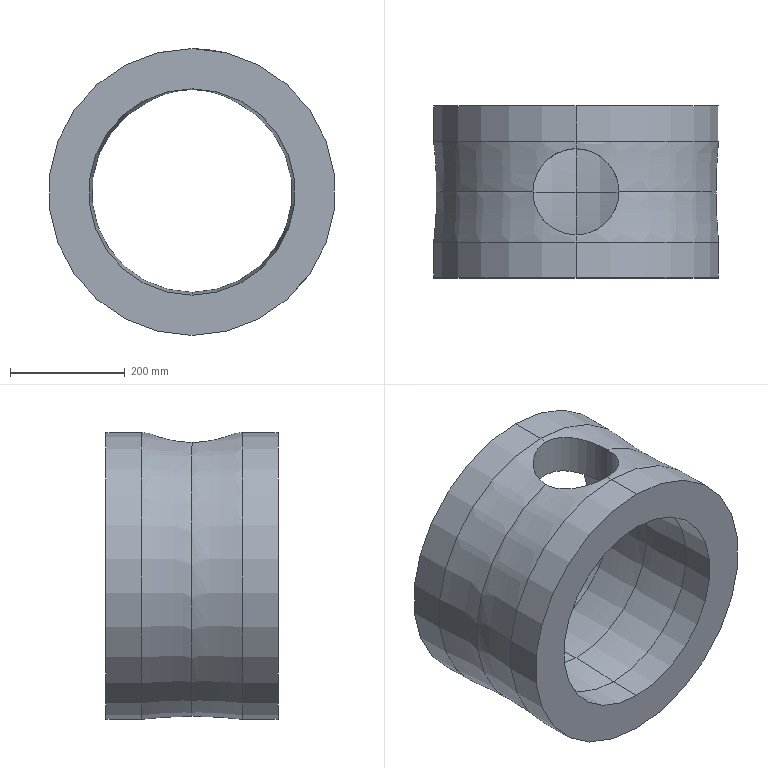Part | SolidWorks | features ICE 1, Revolution 1, Shell 1 | 1 solid | 20 faces | box 500 x 300 x 500 mm | volume 26874622 mm3 | cylinder 10 | torus 8 | plane 2 | commonest cylinder face diameters 360 x4 500 x4 150 x2
STEP:
#1=CARTESIAN_POINT('',(-75.,150.,157.967));
#2=VERTEX_POINT('',#1);
#3=CARTESIAN_POINT('',(0.,225.,178.283));
#4=VERTEX_POINT('',#3);
#5=CARTESIAN_POINT('',(-75.,150.,157.967));
#6=CARTESIAN_POINT('',(-75.,154.992,157.967));
#7=CARTESIAN_POINT('',(-74.507,159.931,158.255));
#8=CARTESIAN_POINT('',(-73.398,165.431,158.877));
#9=CARTESIAN_POINT('',(-73.267,166.041,158.95));
#10=CARTESIAN_POINT('',(-72.99,167.26,159.105));
#11=CARTESIAN_POINT('',(-72.843,167.869,159.186));
#12=CARTESIAN_POINT('',(-72.382,169.683,159.441));
#13=CARTESIAN_POINT('',(-72.046,170.877,159.626));
#14=CARTESIAN_POINT('',(-70.956,174.421,160.219));
#15=CARTESIAN_POINT('',(-70.119,176.728,160.667));
#16=CARTESIAN_POINT('',(-68.229,181.238,161.65));
#17=CARTESIAN_POINT('',(-67.176,183.442,162.186));
#18=CARTESIAN_POINT('',(-65.435,186.671,163.043));
#19=CARTESIAN_POINT('',(-64.826,187.737,163.338));
#20=CARTESIAN_POINT('',(-63.563,189.827,163.939));
#21=CARTESIAN_POINT('',(-62.909,190.852,164.245));
#22=CARTESIAN_POINT('',(-60.881,193.868,165.176));
#23=CARTESIAN_POINT('',(-59.44,195.801,165.814));
#24=CARTESIAN_POINT('',(-56.381,199.518,167.105));
#25=CARTESIAN_POINT('',(-54.763,201.302,167.76));
#26=CARTESIAN_POINT('',(-52.2,203.867,168.74));
#27=CARTESIAN_POINT('',(-51.323,204.703,169.067));
#28=CARTESIAN_POINT('',(-49.521,206.339,169.718));
#29=CARTESIAN_POINT('',(-48.601,207.135,170.041));
#30=CARTESIAN_POINT('',(-45.795,209.445,170.995));
#31=CARTESIAN_POINT('',(-43.859,210.887,171.613));
#32=CARTESIAN_POINT('',(-39.853,213.581,172.796));
#33=CARTESIAN_POINT('',(-37.784,214.833,173.362));
#34=CARTESIAN_POINT('',(-33.507,217.143,174.428));
#35=CARTESIAN_POINT('',(-31.299,218.202,174.928));
#36=CARTESIAN_POINT('',(-28.446,219.399,175.502));
#37=CARTESIAN_POINT('',(-27.87,219.632,175.614));
#38=CARTESIAN_POINT('',(-26.715,220.084,175.833));
#39=CARTESIAN_POINT('',(-26.135,220.302,175.938));
#40=CARTESIAN_POINT('',(-24.391,220.934,176.247));
#41=CARTESIAN_POINT('',(-23.22,221.326,176.439));
#42=CARTESIAN_POINT('',(-19.684,222.413,176.976));
#43=CARTESIAN_POINT('',(-17.296,223.02,177.28));
#44=CARTESIAN_POINT('',(-12.458,223.999,177.773));
#45=CARTESIAN_POINT('',(-10.008,224.371,177.962));
#46=CARTESIAN_POINT('',(-6.284,224.747,178.154));
#47=CARTESIAN_POINT('',(-5.034,224.841,178.202));
#48=CARTESIAN_POINT('',(-3.147,224.937,178.251));
#49=CARTESIAN_POINT('',(-2.516,224.96,178.263));
#50=CARTESIAN_POINT('',(-1.256,224.992,178.279));
#51=CARTESIAN_POINT('',(-0.6274,225.,178.283));
#52=CARTESIAN_POINT('',(0.,225.,178.283));
#53=B_SPLINE_CURVE_WITH_KNOTS('',3,(#5,#6,#7,#8,#9,#10,#11,#12,#13,#14,#15,#16,#17,#18,#19,#20,#21,#22,#23,#24,#25,#26,#27,#28,#29,#30,#31,#32,#33,#34,#35,#36,#37,#38,#39,#40,#41,#42,#43,#44,#45,#46,#47,#48,#49,#50,#51,#52),.UNSPECIFIED.,.F.,.F.,(4,2,2,2,2,2,2,2,2,2,2,2,2,2,2,2,2,2,2,2,2,2,2,4),(0.05661,0.07153,0.0734,0.07526,0.07899,0.08645,0.09392,0.09765,0.1014,0.1088,0.1163,0.12,0.1238,0.1312,0.1387,0.1461,0.148,0.1499,0.1536,0.1611,0.1685,0.1723,0.1741,0.176),.UNSPECIFIED.);
#54=EDGE_CURVE('',#2,#4,#53,.T.);
#55=ORIENTED_EDGE('',*,*,#54,.F.);
#56=CARTESIAN_POINT('',(0.,150.,-174.868));
#57=VERTEX_POINT('',#56);
#58=CARTESIAN_POINT('',(0.,150.,0.));
#59=DIRECTION('',(0.,-1.,0.));
#60=DIRECTION('',(0.,0.,-1.));
#61=AXIS2_PLACEMENT_3D('',#58,#59,#60);
#62=CIRCLE('',#61,174.868);
#63=EDGE_CURVE('',#2,#57,#62,.T.);
#64=ORIENTED_EDGE('',*,*,#63,.T.);
#65=CARTESIAN_POINT('',(0.,241.887,-180.));
#66=VERTEX_POINT('',#65);
#67=CARTESIAN_POINT('',(0.,150.,-1000.));
#68=DIRECTION('',(-1.,0.,0.));
#69=DIRECTION('',(0.,0.,1.));
#70=AXIS2_PLACEMENT_3D('',#67,#68,#69);
#71=CIRCLE('',#70,825.132);
#72=EDGE_CURVE('',#57,#66,#71,.T.);
#73=ORIENTED_EDGE('',*,*,#72,.T.);
#74=CARTESIAN_POINT('',(0.,241.887,180.));
#75=VERTEX_POINT('',#74);
#76=CARTESIAN_POINT('',(0.,241.887,0.));
#77=DIRECTION('',(0.,-1.,0.));
#78=DIRECTION('',(0.,0.,-1.));
#79=AXIS2_PLACEMENT_3D('',#76,#77,#78);
#80=CIRCLE('',#79,180.);
#81=EDGE_CURVE('',#75,#66,#80,.T.);
#82=ORIENTED_EDGE('',*,*,#81,.F.);
#83=CARTESIAN_POINT('',(0.,150.,1000.));
#84=DIRECTION('',(1.,0.,0.));
#85=DIRECTION('',(0.,0.,-1.));
#86=AXIS2_PLACEMENT_3D('',#83,#84,#85);
#87=CIRCLE('',#86,825.132);
#88=EDGE_CURVE('',#4,#75,#87,.T.);
#89=ORIENTED_EDGE('',*,*,#88,.F.);
#90=EDGE_LOOP('',(#55,#64,#73,#82,#89));
#91=FACE_OUTER_BOUND('',#90,.T.);
#92=CARTESIAN_POINT('',(0.,150.,0.));
#93=DIRECTION('',(0.,-1.,0.));
#94=DIRECTION('',(0.,0.,-1.));
#95=AXIS2_PLACEMENT_3D('',#92,#93,#94);
#96=TOROIDAL_SURFACE('',#95,1000.,825.132);
#97=ADVANCED_FACE('',(#91),#96,.T.);
#98=CARTESIAN_POINT('',(0.,62.11,-250.));
#99=VERTEX_POINT('',#98);
#100=CARTESIAN_POINT('',(0.,150.,-244.868));
#101=VERTEX_POINT('',#100);
#102=CARTESIAN_POINT('',(0.,150.,-1000.));
#103=DIRECTION('',(-1.,0.,0.));
#104=DIRECTION('',(0.,0.,1.));
#105=AXIS2_PLACEMENT_3D('',#102,#103,#104);
#106=CIRCLE('',#105,755.132);
#107=EDGE_CURVE('',#99,#101,#106,.T.);
#108=ORIENTED_EDGE('',*,*,#107,.T.);
#109=CARTESIAN_POINT('',(75.,150.,233.099));
#110=VERTEX_POINT('',#109);
#111=CARTESIAN_POINT('',(0.,150.,0.));
#112=DIRECTION('',(0.,-1.,0.));
#113=DIRECTION('',(0.,0.,-1.));
#114=AXIS2_PLACEMENT_3D('',#111,#112,#113);
#115=CIRCLE('',#114,244.868);
#116=EDGE_CURVE('',#101,#110,#115,.T.);
#117=ORIENTED_EDGE('',*,*,#116,.T.);
#118=CARTESIAN_POINT('',(0.,75.,248.601));
#119=VERTEX_POINT('',#118);
#120=CARTESIAN_POINT('',(75.,150.,233.099));
#121=CARTESIAN_POINT('',(75.,148.76,233.099));
#122=CARTESIAN_POINT('',(74.969,147.517,233.112));
#123=CARTESIAN_POINT('',(74.876,145.647,233.152));
#124=CARTESIAN_POINT('',(74.837,145.021,233.168));
#125=CARTESIAN_POINT('',(74.744,143.775,233.208));
#126=CARTESIAN_POINT('',(74.689,143.153,233.231));
#127=CARTESIAN_POINT('',(74.38,140.057,233.362));
#128=CARTESIAN_POINT('',(74.011,137.612,233.518));
#129=CARTESIAN_POINT('',(73.039,132.784,233.923));
#130=CARTESIAN_POINT('',(72.436,130.4,234.172));
#131=CARTESIAN_POINT('',(71.355,126.871,234.61));
#132=CARTESIAN_POINT('',(70.966,125.702,234.767));
#133=CARTESIAN_POINT('',(70.127,123.379,235.1));
#134=CARTESIAN_POINT('',(69.677,122.222,235.278));
#135=CARTESIAN_POINT('',(68.249,118.805,235.834));
#136=CARTESIAN_POINT('',(67.194,116.594,236.237));
#137=CARTESIAN_POINT('',(64.883,112.302,237.092));
#138=CARTESIAN_POINT('',(63.628,110.22,237.544));
#139=CARTESIAN_POINT('',(60.917,106.182,238.484));
#140=CARTESIAN_POINT('',(59.462,104.226,238.973));
#141=CARTESIAN_POINT('',(56.346,100.441,239.972));
#142=CARTESIAN_POINT('',(54.708,98.639,240.477));
#143=CARTESIAN_POINT('',(49.562,93.501,241.979));
#144=CARTESIAN_POINT('',(45.825,90.427,242.968));
#145=CARTESIAN_POINT('',(40.75,87.024,244.122));
#146=CARTESIAN_POINT('',(39.714,86.366,244.35));
#147=CARTESIAN_POINT('',(37.604,85.097,244.793));
#148=CARTESIAN_POINT('',(36.537,84.49,245.008));
#149=CARTESIAN_POINT('',(33.301,82.754,245.63));
#150=CARTESIAN_POINT('',(31.097,81.707,246.015));
#151=CARTESIAN_POINT('',(26.593,79.83,246.716));
#152=CARTESIAN_POINT('',(24.293,79.001,247.032));
#153=CARTESIAN_POINT('',(19.596,77.564,247.587));
#154=CARTESIAN_POINT('',(17.198,76.956,247.825));
#155=CARTESIAN_POINT('',(9.852,75.482,248.406));
#156=CARTESIAN_POINT('',(4.935,75.,248.601));
#157=CARTESIAN_POINT('',(0.,75.,248.601));
#158=B_SPLINE_CURVE_WITH_KNOTS('',3,(#120,#121,#122,#123,#124,#125,#126,#127,#128,#129,#130,#131,#132,#133,#134,#135,#136,#137,#138,#139,#140,#141,#142,#143,#144,#145,#146,#147,#148,#149,#150,#151,#152,#153,#154,#155,#156,#157),.UNSPECIFIED.,.F.,.F.,(4,2,2,2,2,2,2,2,2,2,2,2,2,2,2,2,2,2,4),(0.2931,0.2968,0.2986,0.3005,0.3079,0.3153,0.319,0.3227,0.3301,0.3375,0.3449,0.3523,0.3671,0.3708,0.3745,0.3819,0.3893,0.3967,0.4115),.UNSPECIFIED.);
#159=EDGE_CURVE('',#110,#119,#158,.T.);
#160=ORIENTED_EDGE('',*,*,#159,.T.);
#161=CARTESIAN_POINT('',(0.,62.11,250.));
#162=VERTEX_POINT('',#161);
#163=CARTESIAN_POINT('',(0.,150.,1000.));
#164=DIRECTION('',(1.,0.,0.));
#165=DIRECTION('',(0.,0.,-1.));
#166=AXIS2_PLACEMENT_3D('',#163,#164,#165);
#167=CIRCLE('',#166,755.132);
#168=EDGE_CURVE('',#162,#119,#167,.T.);
#169=ORIENTED_EDGE('',*,*,#168,.F.);
#170=CARTESIAN_POINT('',(0.,62.11,0.));
#171=DIRECTION('',(0.,-1.,0.));
#172=DIRECTION('',(0.,0.,-1.));
#173=AXIS2_PLACEMENT_3D('',#170,#171,#172);
#174=CIRCLE('',#173,250.);
#175=EDGE_CURVE('',#99,#162,#174,.T.);
#176=ORIENTED_EDGE('',*,*,#175,.F.);
#177=EDGE_LOOP('',(#108,#117,#160,#169,#176));
#178=FACE_OUTER_BOUND('',#177,.T.);
#179=CARTESIAN_POINT('',(0.,150.,0.));
#180=DIRECTION('',(0.,-1.,0.));
#181=DIRECTION('',(0.,0.,-1.));
#182=AXIS2_PLACEMENT_3D('',#179,#180,#181);
#183=TOROIDAL_SURFACE('',#182,1000.,755.132);
#184=ADVANCED_FACE('',(#178),#183,.F.);
#185=CARTESIAN_POINT('',(-75.,150.,233.099));
#186=VERTEX_POINT('',#185);
#187=CARTESIAN_POINT('',(0.,75.,248.601));
#188=CARTESIAN_POINT('',(-2.466,75.,248.601));
#189=CARTESIAN_POINT('',(-4.938,75.121,248.553));
#190=CARTESIAN_POINT('',(-8.652,75.49,248.405));
#191=CARTESIAN_POINT('',(-9.895,75.645,248.343));
#192=CARTESIAN_POINT('',(-12.36,76.015,248.196));
#193=CARTESIAN_POINT('',(-13.582,76.23,248.111));
#194=CARTESIAN_POINT('',(-19.644,77.449,247.63));
#195=CARTESIAN_POINT('',(-24.337,78.888,247.068));
#196=CARTESIAN_POINT('',(-30.014,81.256,246.183));
#197=CARTESIAN_POINT('',(-31.14,81.759,245.997));
#198=CARTESIAN_POINT('',(-33.372,82.822,245.607));
#199=CARTESIAN_POINT('',(-34.469,83.379,245.406));
#200=CARTESIAN_POINT('',(-37.706,85.121,244.782));
#201=CARTESIAN_POINT('',(-39.791,86.38,244.341));
#202=CARTESIAN_POINT('',(-43.823,89.087,243.423));
#203=CARTESIAN_POINT('',(-45.77,90.535,242.945));
#204=CARTESIAN_POINT('',(-48.586,92.852,242.21));
#205=CARTESIAN_POINT('',(-49.508,93.648,241.962));
#206=CARTESIAN_POINT('',(-51.316,95.29,241.461));
#207=CARTESIAN_POINT('',(-52.204,96.136,241.208));
#208=CARTESIAN_POINT('',(-53.934,97.869,240.702));
#209=CARTESIAN_POINT('',(-54.779,98.758,240.448));
#210=CARTESIAN_POINT('',(-56.42,100.571,239.944));
#211=CARTESIAN_POINT('',(-57.216,101.494,239.694));
#212=CARTESIAN_POINT('',(-59.529,104.314,238.951));
#213=CARTESIAN_POINT('',(-60.972,106.259,238.466));
#214=CARTESIAN_POINT('',(-63.667,110.284,237.53));
#215=CARTESIAN_POINT('',(-64.918,112.363,237.079));
#216=CARTESIAN_POINT('',(-66.649,115.584,236.438));
#217=CARTESIAN_POINT('',(-67.201,116.675,236.231));
#218=CARTESIAN_POINT('',(-68.256,118.893,235.83));
#219=CARTESIAN_POINT('',(-68.76,120.023,235.635));
#220=CARTESIAN_POINT('',(-71.131,125.715,234.711));
#221=CARTESIAN_POINT('',(-72.56,130.4,234.123));
#222=CARTESIAN_POINT('',(-74.013,137.625,233.517));
#223=CARTESIAN_POINT('',(-74.381,140.066,233.362));
#224=CARTESIAN_POINT('',(-74.752,143.781,233.205));
#225=CARTESIAN_POINT('',(-74.846,145.031,233.165));
#226=CARTESIAN_POINT('',(-74.969,147.521,233.112));
#227=CARTESIAN_POINT('',(-75.,148.762,233.099));
#228=CARTESIAN_POINT('',(-75.,150.,233.099));
#229=B_SPLINE_CURVE_WITH_KNOTS('',3,(#187,#188,#189,#190,#191,#192,#193,#194,#195,#196,#197,#198,#199,#200,#201,#202,#203,#204,#205,#206,#207,#208,#209,#210,#211,#212,#213,#214,#215,#216,#217,#218,#219,#220,#221,#222,#223,#224,#225,#226,#227,#228),.UNSPECIFIED.,.F.,.F.,(4,2,2,2,2,2,2,2,2,2,2,2,2,2,2,2,2,2,2,2,4),(0.4115,0.4189,0.4226,0.4263,0.4411,0.4448,0.4485,0.4559,0.4633,0.467,0.4707,0.4744,0.4781,0.4855,0.4929,0.4966,0.5003,0.5151,0.5225,0.5262,0.5299),.UNSPECIFIED.);
#230=EDGE_CURVE('',#119,#186,#229,.T.);
#231=ORIENTED_EDGE('',*,*,#230,.T.);
#232=CARTESIAN_POINT('',(0.,150.,0.));
#233=DIRECTION('',(0.,-1.,0.));
#234=DIRECTION('',(0.,0.,-1.));
#235=AXIS2_PLACEMENT_3D('',#232,#233,#234);
#236=CIRCLE('',#235,244.868);
#237=EDGE_CURVE('',#186,#101,#236,.T.);
#238=ORIENTED_EDGE('',*,*,#237,.T.);
#239=ORIENTED_EDGE('',*,*,#107,.F.);
#240=CARTESIAN_POINT('',(0.,62.11,0.));
#241=DIRECTION('',(0.,-1.,0.));
#242=DIRECTION('',(0.,0.,-1.));
#243=AXIS2_PLACEMENT_3D('',#240,#241,#242);
#244=CIRCLE('',#243,250.);
#245=EDGE_CURVE('',#162,#99,#244,.T.);
#246=ORIENTED_EDGE('',*,*,#245,.F.);
#247=ORIENTED_EDGE('',*,*,#168,.T.);
#248=EDGE_LOOP('',(#231,#238,#239,#246,#247));
#249=FACE_OUTER_BOUND('',#248,.T.);
#250=CARTESIAN_POINT('',(0.,150.,0.));
#251=DIRECTION('',(0.,-1.,0.));
#252=DIRECTION('',(0.,0.,-1.));
#253=AXIS2_PLACEMENT_3D('',#250,#251,#252);
#254=TOROIDAL_SURFACE('',#253,1000.,755.132);
#255=ADVANCED_FACE('',(#249),#254,.F.);
#256=ORIENTED_EDGE('',*,*,#72,.F.);
#257=CARTESIAN_POINT('',(75.,150.,157.967));
#258=VERTEX_POINT('',#257);
#259=CARTESIAN_POINT('',(0.,150.,0.));
#260=DIRECTION('',(0.,-1.,0.));
#261=DIRECTION('',(0.,0.,-1.));
#262=AXIS2_PLACEMENT_3D('',#259,#260,#261);
#263=CIRCLE('',#262,174.868);
#264=EDGE_CURVE('',#57,#258,#263,.T.);
#265=ORIENTED_EDGE('',*,*,#264,.T.);
#266=CARTESIAN_POINT('',(0.,225.,178.283));
#267=CARTESIAN_POINT('',(5.018,225.,178.283));
#268=CARTESIAN_POINT('',(9.963,224.501,178.026));
#269=CARTESIAN_POINT('',(16.056,223.272,177.407));
#270=CARTESIAN_POINT('',(17.27,222.995,177.268));
#271=CARTESIAN_POINT('',(19.689,222.38,176.961));
#272=CARTESIAN_POINT('',(20.896,222.041,176.792));
#273=CARTESIAN_POINT('',(24.462,220.942,176.25));
#274=CARTESIAN_POINT('',(26.779,220.099,175.838));
#275=CARTESIAN_POINT('',(31.301,218.2,174.927));
#276=CARTESIAN_POINT('',(33.505,217.145,174.428));
#277=CARTESIAN_POINT('',(36.728,215.403,173.625));
#278=CARTESIAN_POINT('',(37.789,214.796,173.348));
#279=CARTESIAN_POINT('',(39.883,213.528,172.776));
#280=CARTESIAN_POINT('',(40.919,212.866,172.482));
#281=CARTESIAN_POINT('',(43.955,210.819,171.583));
#282=CARTESIAN_POINT('',(45.895,209.368,170.963));
#283=CARTESIAN_POINT('',(49.614,206.296,169.696));
#284=CARTESIAN_POINT('',(51.394,204.676,169.049));
#285=CARTESIAN_POINT('',(54.797,201.265,167.746));
#286=CARTESIAN_POINT('',(56.421,199.473,167.089));
#287=CARTESIAN_POINT('',(58.738,196.651,166.11));
#288=CARTESIAN_POINT('',(59.486,195.693,165.786));
#289=CARTESIAN_POINT('',(60.931,193.748,165.148));
#290=CARTESIAN_POINT('',(61.628,192.761,164.833));
#291=CARTESIAN_POINT('',(63.645,189.752,163.907));
#292=CARTESIAN_POINT('',(64.89,187.685,163.311));
#293=CARTESIAN_POINT('',(67.184,183.424,162.182));
#294=CARTESIAN_POINT('',(68.233,181.23,161.648));
#295=CARTESIAN_POINT('',(69.653,177.838,160.909));
#296=CARTESIAN_POINT('',(70.101,176.691,160.673));
#297=CARTESIAN_POINT('',(70.733,174.943,160.336));
#298=CARTESIAN_POINT('',(70.938,174.355,160.226));
#299=CARTESIAN_POINT('',(71.331,173.178,160.014));
#300=CARTESIAN_POINT('',(71.521,172.587,159.912));
#301=CARTESIAN_POINT('',(72.429,169.628,159.418));
#302=CARTESIAN_POINT('',(73.035,167.235,159.081));
#303=CARTESIAN_POINT('',(74.009,162.399,158.534));
#304=CARTESIAN_POINT('',(74.378,159.956,158.324));
#305=CARTESIAN_POINT('',(74.873,155.018,158.041));
#306=CARTESIAN_POINT('',(75.,152.523,157.967));
#307=CARTESIAN_POINT('',(75.,150.,157.967));
#308=B_SPLINE_CURVE_WITH_KNOTS('',3,(#266,#267,#268,#269,#270,#271,#272,#273,#274,#275,#276,#277,#278,#279,#280,#281,#282,#283,#284,#285,#286,#287,#288,#289,#290,#291,#292,#293,#294,#295,#296,#297,#298,#299,#300,#301,#302,#303,#304,#305,#306,#307),.UNSPECIFIED.,.F.,.F.,(4,2,2,2,2,2,2,2,2,2,2,2,2,2,2,2,2,2,2,2,4),(0.176,0.1909,0.1946,0.1984,0.2058,0.2133,0.217,0.2207,0.2282,0.2357,0.2431,0.2469,0.2506,0.258,0.2655,0.2692,0.2711,0.273,0.2804,0.2879,0.2953),.UNSPECIFIED.);
#309=EDGE_CURVE('',#4,#258,#308,.T.);
#310=ORIENTED_EDGE('',*,*,#309,.F.);
#311=ORIENTED_EDGE('',*,*,#88,.T.);
#312=CARTESIAN_POINT('',(0.,241.887,0.));
#313=DIRECTION('',(0.,-1.,0.));
#314=DIRECTION('',(0.,0.,-1.));
#315=AXIS2_PLACEMENT_3D('',#312,#313,#314);
#316=CIRCLE('',#315,180.);
#317=EDGE_CURVE('',#66,#75,#316,.T.);
#318=ORIENTED_EDGE('',*,*,#317,.F.);
#319=EDGE_LOOP('',(#256,#265,#310,#311,#318));
#320=FACE_OUTER_BOUND('',#319,.T.);
#321=CARTESIAN_POINT('',(0.,150.,0.));
#322=DIRECTION('',(0.,-1.,0.));
#323=DIRECTION('',(0.,0.,-1.));
#324=AXIS2_PLACEMENT_3D('',#321,#322,#323);
#325=TOROIDAL_SURFACE('',#324,1000.,825.132);
#326=ADVANCED_FACE('',(#320),#325,.T.);
#327=ORIENTED_EDGE('',*,*,#159,.F.);
#328=CARTESIAN_POINT('',(75.,150.,689.));
#329=DIRECTION('',(0.,0.,-1.));
#330=VECTOR('',#329,1000.);
#331=LINE('',#328,#330);
#332=EDGE_CURVE('',#110,#258,#331,.T.);
#333=ORIENTED_EDGE('',*,*,#332,.T.);
#334=CARTESIAN_POINT('',(0.,75.,178.283));
#335=VERTEX_POINT('',#334);
#336=CARTESIAN_POINT('',(75.,150.,157.967));
#337=CARTESIAN_POINT('',(75.,149.37,157.967));
#338=CARTESIAN_POINT('',(74.992,148.738,157.972));
#339=CARTESIAN_POINT('',(74.96,147.479,157.99));
#340=CARTESIAN_POINT('',(74.937,146.852,158.004));
#341=CARTESIAN_POINT('',(74.842,144.974,158.058));
#342=CARTESIAN_POINT('',(74.748,143.728,158.112));
#343=CARTESIAN_POINT('',(74.374,140.012,158.326));
#344=CARTESIAN_POINT('',(74.003,137.56,158.538));
#345=CARTESIAN_POINT('',(73.021,132.707,159.088));
#346=CARTESIAN_POINT('',(72.411,130.305,159.428));
#347=CARTESIAN_POINT('',(71.496,127.334,159.925));
#348=CARTESIAN_POINT('',(71.305,126.741,160.028));
#349=CARTESIAN_POINT('',(70.91,125.564,160.241));
#350=CARTESIAN_POINT('',(70.706,124.98,160.35));
#351=CARTESIAN_POINT('',(70.074,123.239,160.687));
#352=CARTESIAN_POINT('',(69.626,122.094,160.923));
#353=CARTESIAN_POINT('',(68.203,118.706,161.663));
#354=CARTESIAN_POINT('',(67.151,116.509,162.199));
#355=CARTESIAN_POINT('',(64.842,112.231,163.335));
#356=CARTESIAN_POINT('',(63.584,110.151,163.935));
#357=CARTESIAN_POINT('',(61.542,107.116,164.872));
#358=CARTESIAN_POINT('',(60.836,106.12,165.19));
#359=CARTESIAN_POINT('',(59.386,104.176,165.83));
#360=CARTESIAN_POINT('',(58.639,103.225,166.152));
#361=CARTESIAN_POINT('',(56.338,100.434,167.123));
#362=CARTESIAN_POINT('',(54.722,98.655,167.776));
#363=CARTESIAN_POINT('',(51.32,95.255,169.076));
#364=CARTESIAN_POINT('',(49.536,93.635,169.724));
#365=CARTESIAN_POINT('',(46.729,91.324,170.678));
#366=CARTESIAN_POINT('',(45.77,90.573,170.993));
#367=CARTESIAN_POINT('',(43.811,89.114,171.616));
#368=CARTESIAN_POINT('',(42.817,88.411,171.921));
#369=CARTESIAN_POINT('',(37.774,85.025,173.409));
#370=CARTESIAN_POINT('',(33.507,82.723,174.484));
#371=CARTESIAN_POINT('',(26.739,79.886,175.845));
#372=CARTESIAN_POINT('',(24.422,79.044,176.256));
#373=CARTESIAN_POINT('',(21.441,78.127,176.709));
#374=CARTESIAN_POINT('',(20.841,77.951,176.796));
#375=CARTESIAN_POINT('',(19.64,77.614,176.963));
#376=CARTESIAN_POINT('',(19.038,77.454,177.043));
#377=CARTESIAN_POINT('',(17.229,76.995,177.272));
#378=CARTESIAN_POINT('',(16.019,76.72,177.411));
#379=CARTESIAN_POINT('',(9.944,75.497,178.027));
#380=CARTESIAN_POINT('',(5.01,75.,178.283));
#381=CARTESIAN_POINT('',(0.,75.,178.283));
#382=B_SPLINE_CURVE_WITH_KNOTS('',3,(#336,#337,#338,#339,#340,#341,#342,#343,#344,#345,#346,#347,#348,#349,#350,#351,#352,#353,#354,#355,#356,#357,#358,#359,#360,#361,#362,#363,#364,#365,#366,#367,#368,#369,#370,#371,#372,#373,#374,#375,#376,#377,#378,#379,#380,#381),.UNSPECIFIED.,.F.,.F.,(4,2,2,2,2,2,2,2,2,2,2,2,2,2,2,2,2,2,2,2,2,2,4),(0.2953,0.2972,0.2991,0.3028,0.3103,0.3177,0.3196,0.3214,0.3252,0.3326,0.3401,0.3438,0.3475,0.355,0.3624,0.3662,0.3699,0.3848,0.3922,0.3941,0.396,0.3997,0.4146),.UNSPECIFIED.);
#383=EDGE_CURVE('',#258,#335,#382,.T.);
#384=ORIENTED_EDGE('',*,*,#383,.T.);
#385=CARTESIAN_POINT('',(0.,75.,178.283));
#386=CARTESIAN_POINT('',(-1.251,75.,178.283));
#387=CARTESIAN_POINT('',(-2.509,75.031,178.267));
#388=CARTESIAN_POINT('',(-5.028,75.158,178.202));
#389=CARTESIAN_POINT('',(-6.279,75.253,178.154));
#390=CARTESIAN_POINT('',(-10.009,75.629,177.962));
#391=CARTESIAN_POINT('',(-12.466,76.002,177.773));
#392=CARTESIAN_POINT('',(-17.319,76.985,177.277));
#393=CARTESIAN_POINT('',(-19.717,77.596,176.971));
#394=CARTESIAN_POINT('',(-23.268,78.69,176.431));
#395=CARTESIAN_POINT('',(-24.445,79.085,176.237));
#396=CARTESIAN_POINT('',(-26.783,79.934,175.824));
#397=CARTESIAN_POINT('',(-27.936,80.386,175.605));
#398=CARTESIAN_POINT('',(-31.342,81.818,174.918));
#399=CARTESIAN_POINT('',(-33.546,82.876,174.419));
#400=CARTESIAN_POINT('',(-37.828,85.193,173.35));
#401=CARTESIAN_POINT('',(-39.905,86.451,172.781));
#402=CARTESIAN_POINT('',(-42.929,88.489,171.887));
#403=CARTESIAN_POINT('',(-43.922,89.194,171.582));
#404=CARTESIAN_POINT('',(-45.876,90.654,170.959));
#405=CARTESIAN_POINT('',(-46.835,91.408,170.643));
#406=CARTESIAN_POINT('',(-49.646,93.731,169.684));
#407=CARTESIAN_POINT('',(-51.439,95.365,169.033));
#408=CARTESIAN_POINT('',(-54.007,97.945,168.048));
#409=CARTESIAN_POINT('',(-54.845,98.829,167.718));
#410=CARTESIAN_POINT('',(-56.47,100.628,167.062));
#411=CARTESIAN_POINT('',(-57.257,101.543,166.736));
#412=CARTESIAN_POINT('',(-59.549,104.341,165.766));
#413=CARTESIAN_POINT('',(-60.981,106.272,165.131));
#414=CARTESIAN_POINT('',(-63.657,110.268,163.901));
#415=CARTESIAN_POINT('',(-64.901,112.334,163.306));
#416=CARTESIAN_POINT('',(-66.625,115.539,162.457));
#417=CARTESIAN_POINT('',(-67.176,116.625,162.181));
#418=CARTESIAN_POINT('',(-68.229,118.834,161.647));
#419=CARTESIAN_POINT('',(-68.732,119.96,161.388));
#420=CARTESIAN_POINT('',(-71.102,125.633,160.154));
#421=CARTESIAN_POINT('',(-72.537,130.313,159.36));
#422=CARTESIAN_POINT('',(-74.001,137.555,158.538));
#423=CARTESIAN_POINT('',(-74.373,140.006,158.326));
#424=CARTESIAN_POINT('',(-74.749,143.743,158.112));
#425=CARTESIAN_POINT('',(-74.844,145.002,158.057));
#426=CARTESIAN_POINT('',(-74.969,147.506,157.985));
#427=CARTESIAN_POINT('',(-75.,148.755,157.967));
#428=CARTESIAN_POINT('',(-75.,150.,157.967));
#429=B_SPLINE_CURVE_WITH_KNOTS('',3,(#385,#386,#387,#388,#389,#390,#391,#392,#393,#394,#395,#396,#397,#398,#399,#400,#401,#402,#403,#404,#405,#406,#407,#408,#409,#410,#411,#412,#413,#414,#415,#416,#417,#418,#419,#420,#421,#422,#423,#424,#425,#426,#427,#428),.UNSPECIFIED.,.F.,.F.,(4,2,2,2,2,2,2,2,2,2,2,2,2,2,2,2,2,2,2,2,2,4),(0.4146,0.4183,0.422,0.4295,0.4369,0.4407,0.4444,0.4518,0.4593,0.463,0.4667,0.4742,0.4779,0.4816,0.4891,0.4965,0.5002,0.504,0.5188,0.5263,0.53,0.5337),.UNSPECIFIED.);
#430=EDGE_CURVE('',#335,#2,#429,.T.);
#431=ORIENTED_EDGE('',*,*,#430,.T.);
#432=CARTESIAN_POINT('',(-75.,150.,689.));
#433=DIRECTION('',(0.,0.,-1.));
#434=VECTOR('',#433,1000.);
#435=LINE('',#432,#434);
#436=EDGE_CURVE('',#186,#2,#435,.T.);
#437=ORIENTED_EDGE('',*,*,#436,.F.);
#438=ORIENTED_EDGE('',*,*,#230,.F.);
#439=EDGE_LOOP('',(#327,#333,#384,#431,#437,#438));
#440=FACE_OUTER_BOUND('',#439,.T.);
#441=CARTESIAN_POINT('',(0.,150.,689.));
#442=DIRECTION('',(0.,0.,-1.));
#443=DIRECTION('',(-1.,0.,0.));
#444=AXIS2_PLACEMENT_3D('',#441,#442,#443);
#445=CYLINDRICAL_SURFACE('',#444,75.);
#446=ADVANCED_FACE('',(#440),#445,.F.);
#447=CARTESIAN_POINT('',(0.,300.,180.));
#448=VERTEX_POINT('',#447);
#449=CARTESIAN_POINT('',(0.,300.,-180.));
#450=VERTEX_POINT('',#449);
#451=CARTESIAN_POINT('',(0.,300.,0.));
#452=DIRECTION('',(0.,-1.,0.));
#453=DIRECTION('',(0.,0.,1.));
#454=AXIS2_PLACEMENT_3D('',#451,#452,#453);
#455=CIRCLE('',#454,180.);
#456=EDGE_CURVE('',#448,#450,#455,.T.);
#457=ORIENTED_EDGE('',*,*,#456,.F.);
#458=CARTESIAN_POINT('',(0.,0.,180.));
#459=DIRECTION('',(0.,-1.,0.));
#460=VECTOR('',#459,1000.);
#461=LINE('',#458,#460);
#462=EDGE_CURVE('',#448,#75,#461,.T.);
#463=ORIENTED_EDGE('',*,*,#462,.T.);
#464=ORIENTED_EDGE('',*,*,#81,.T.);
#465=CARTESIAN_POINT('',(0.,0.,-180.));
#466=DIRECTION('',(0.,-1.,0.));
#467=VECTOR('',#466,1000.);
#468=LINE('',#465,#467);
#469=EDGE_CURVE('',#450,#66,#468,.T.);
#470=ORIENTED_EDGE('',*,*,#469,.F.);
#471=EDGE_LOOP('',(#457,#463,#464,#470));
#472=FACE_OUTER_BOUND('',#471,.T.);
#473=CARTESIAN_POINT('',(0.,0.,0.));
#474=DIRECTION('',(0.,-1.,0.));
#475=DIRECTION('',(0.,0.,-1.));
#476=AXIS2_PLACEMENT_3D('',#473,#474,#475);
#477=CYLINDRICAL_SURFACE('',#476,180.);
#478=ADVANCED_FACE('',(#472),#477,.F.);
#479=CARTESIAN_POINT('',(0.,58.113,180.));
#480=VERTEX_POINT('',#479);
#481=CARTESIAN_POINT('',(0.,58.113,-180.));
#482=VERTEX_POINT('',#481);
#483=CARTESIAN_POINT('',(0.,58.113,0.));
#484=DIRECTION('',(0.,-1.,0.));
#485=DIRECTION('',(0.,0.,1.));
#486=AXIS2_PLACEMENT_3D('',#483,#484,#485);
#487=CIRCLE('',#486,180.);
#488=EDGE_CURVE('',#480,#482,#487,.T.);
#489=ORIENTED_EDGE('',*,*,#488,.F.);
#490=CARTESIAN_POINT('',(0.,0.,180.));
#491=VERTEX_POINT('',#490);
#492=CARTESIAN_POINT('',(0.,0.,180.));
#493=DIRECTION('',(0.,-1.,0.));
#494=VECTOR('',#493,1000.);
#495=LINE('',#492,#494);
#496=EDGE_CURVE('',#480,#491,#495,.T.);
#497=ORIENTED_EDGE('',*,*,#496,.T.);
#498=CARTESIAN_POINT('',(0.,0.,-180.));
#499=VERTEX_POINT('',#498);
#500=CARTESIAN_POINT('',(0.,0.,0.));
#501=DIRECTION('',(0.,-1.,0.));
#502=DIRECTION('',(0.,0.,-1.));
#503=AXIS2_PLACEMENT_3D('',#500,#501,#502);
#504=CIRCLE('',#503,180.);
#505=EDGE_CURVE('',#491,#499,#504,.T.);
#506=ORIENTED_EDGE('',*,*,#505,.T.);
#507=CARTESIAN_POINT('',(0.,0.,-180.));
#508=DIRECTION('',(0.,-1.,0.));
#509=VECTOR('',#508,1000.);
#510=LINE('',#507,#509);
#511=EDGE_CURVE('',#482,#499,#510,.T.);
#512=ORIENTED_EDGE('',*,*,#511,.F.);
#513=EDGE_LOOP('',(#489,#497,#506,#512));
#514=FACE_OUTER_BOUND('',#513,.T.);
#515=CARTESIAN_POINT('',(0.,0.,0.));
#516=DIRECTION('',(0.,-1.,0.));
#517=DIRECTION('',(0.,0.,-1.));
#518=AXIS2_PLACEMENT_3D('',#515,#516,#517);
#519=CYLINDRICAL_SURFACE('',#518,180.);
#520=ADVANCED_FACE('',(#514),#519,.F.);
#521=CARTESIAN_POINT('',(0.,300.,-250.));
#522=VERTEX_POINT('',#521);
#523=CARTESIAN_POINT('',(0.,300.,250.));
#524=VERTEX_POINT('',#523);
#525=CARTESIAN_POINT('',(0.,300.,0.));
#526=DIRECTION('',(0.,-1.,0.));
#527=DIRECTION('',(0.,0.,-1.));
#528=AXIS2_PLACEMENT_3D('',#525,#526,#527);
#529=CIRCLE('',#528,250.);
#530=EDGE_CURVE('',#522,#524,#529,.T.);
#531=ORIENTED_EDGE('',*,*,#530,.T.);
#532=CARTESIAN_POINT('',(0.,237.89,250.));
#533=VERTEX_POINT('',#532);
#534=CARTESIAN_POINT('',(0.,0.,250.));
#535=DIRECTION('',(0.,-1.,0.));
#536=VECTOR('',#535,1000.);
#537=LINE('',#534,#536);
#538=EDGE_CURVE('',#524,#533,#537,.T.);
#539=ORIENTED_EDGE('',*,*,#538,.T.);
#540=CARTESIAN_POINT('',(0.,237.89,-250.));
#541=VERTEX_POINT('',#540);
#542=CARTESIAN_POINT('',(0.,237.89,0.));
#543=DIRECTION('',(0.,-1.,0.));
#544=DIRECTION('',(0.,0.,-1.));
#545=AXIS2_PLACEMENT_3D('',#542,#543,#544);
#546=CIRCLE('',#545,250.);
#547=EDGE_CURVE('',#541,#533,#546,.T.);
#548=ORIENTED_EDGE('',*,*,#547,.F.);
#549=CARTESIAN_POINT('',(0.,0.,-250.));
#550=DIRECTION('',(0.,-1.,0.));
#551=VECTOR('',#550,1000.);
#552=LINE('',#549,#551);
#553=EDGE_CURVE('',#522,#541,#552,.T.);
#554=ORIENTED_EDGE('',*,*,#553,.F.);
#555=EDGE_LOOP('',(#531,#539,#548,#554));
#556=FACE_OUTER_BOUND('',#555,.T.);
#557=CARTESIAN_POINT('',(0.,0.,0.));
#558=DIRECTION('',(0.,-1.,0.));
#559=DIRECTION('',(0.,0.,-1.));
#560=AXIS2_PLACEMENT_3D('',#557,#558,#559);
#561=CYLINDRICAL_SURFACE('',#560,250.);
#562=ADVANCED_FACE('',(#556),#561,.T.);
#563=ORIENTED_EDGE('',*,*,#175,.T.);
#564=CARTESIAN_POINT('',(0.,0.,250.));
#565=VERTEX_POINT('',#564);
#566=CARTESIAN_POINT('',(0.,0.,250.));
#567=DIRECTION('',(0.,-1.,0.));
#568=VECTOR('',#567,1000.);
#569=LINE('',#566,#568);
#570=EDGE_CURVE('',#162,#565,#569,.T.);
#571=ORIENTED_EDGE('',*,*,#570,.T.);
#572=CARTESIAN_POINT('',(0.,0.,-250.));
#573=VERTEX_POINT('',#572);
#574=CARTESIAN_POINT('',(0.,0.,0.));
#575=DIRECTION('',(0.,-1.,0.));
#576=DIRECTION('',(0.,0.,-1.));
#577=AXIS2_PLACEMENT_3D('',#574,#575,#576);
#578=CIRCLE('',#577,250.);
#579=EDGE_CURVE('',#573,#565,#578,.T.);
#580=ORIENTED_EDGE('',*,*,#579,.F.);
#581=CARTESIAN_POINT('',(0.,0.,-250.));
#582=DIRECTION('',(0.,-1.,0.));
#583=VECTOR('',#582,1000.);
#584=LINE('',#581,#583);
#585=EDGE_CURVE('',#99,#573,#584,.T.);
#586=ORIENTED_EDGE('',*,*,#585,.F.);
#587=EDGE_LOOP('',(#563,#571,#580,#586));
#588=FACE_OUTER_BOUND('',#587,.T.);
#589=CARTESIAN_POINT('',(0.,0.,0.));
#590=DIRECTION('',(0.,-1.,0.));
#591=DIRECTION('',(0.,0.,-1.));
#592=AXIS2_PLACEMENT_3D('',#589,#590,#591);
#593=CYLINDRICAL_SURFACE('',#592,250.);
#594=ADVANCED_FACE('',(#588),#593,.T.);
#595=ORIENTED_EDGE('',*,*,#264,.F.);
#596=CARTESIAN_POINT('',(0.,150.,-1000.));
#597=DIRECTION('',(-1.,0.,0.));
#598=DIRECTION('',(0.,0.,1.));
#599=AXIS2_PLACEMENT_3D('',#596,#597,#598);
#600=CIRCLE('',#599,825.132);
#601=EDGE_CURVE('',#482,#57,#600,.T.);
#602=ORIENTED_EDGE('',*,*,#601,.F.);
#603=CARTESIAN_POINT('',(0.,58.113,0.));
#604=DIRECTION('',(0.,-1.,0.));
#605=DIRECTION('',(0.,0.,1.));
#606=AXIS2_PLACEMENT_3D('',#603,#604,#605);
#607=CIRCLE('',#606,180.);
#608=EDGE_CURVE('',#482,#480,#607,.T.);
#609=ORIENTED_EDGE('',*,*,#608,.T.);
#610=CARTESIAN_POINT('',(0.,150.,1000.));
#611=DIRECTION('',(1.,0.,0.));
#612=DIRECTION('',(0.,0.,-1.));
#613=AXIS2_PLACEMENT_3D('',#610,#611,#612);
#614=CIRCLE('',#613,825.132);
#615=EDGE_CURVE('',#480,#335,#614,.T.);
#616=ORIENTED_EDGE('',*,*,#615,.T.);
#617=ORIENTED_EDGE('',*,*,#383,.F.);
#618=EDGE_LOOP('',(#595,#602,#609,#616,#617));
#619=FACE_OUTER_BOUND('',#618,.T.);
#620=CARTESIAN_POINT('',(0.,150.,0.));
#621=DIRECTION('',(0.,-1.,0.));
#622=DIRECTION('',(0.,0.,-1.));
#623=AXIS2_PLACEMENT_3D('',#620,#621,#622);
#624=TOROIDAL_SURFACE('',#623,1000.,825.132);
#625=ADVANCED_FACE('',(#619),#624,.T.);
#626=ORIENTED_EDGE('',*,*,#237,.F.);
#627=CARTESIAN_POINT('',(0.,225.,248.601));
#628=VERTEX_POINT('',#627);
#629=CARTESIAN_POINT('',(-75.,150.,233.099));
#630=CARTESIAN_POINT('',(-75.,154.959,233.099));
#631=CARTESIAN_POINT('',(-74.513,159.868,233.309));
#632=CARTESIAN_POINT('',(-73.297,165.942,233.816));
#633=CARTESIAN_POINT('',(-73.023,167.153,233.929));
#634=CARTESIAN_POINT('',(-72.412,169.57,234.181));
#635=CARTESIAN_POINT('',(-72.079,170.765,234.317));
#636=CARTESIAN_POINT('',(-70.994,174.308,234.756));
#637=CARTESIAN_POINT('',(-70.161,176.617,235.089));
#638=CARTESIAN_POINT('',(-68.277,181.131,235.823));
#639=CARTESIAN_POINT('',(-67.228,183.338,236.224));
#640=CARTESIAN_POINT('',(-65.491,186.571,236.867));
#641=CARTESIAN_POINT('',(-64.885,187.636,237.088));
#642=CARTESIAN_POINT('',(-63.618,189.74,237.543));
#643=CARTESIAN_POINT('',(-62.957,190.779,237.777));
#644=CARTESIAN_POINT('',(-59.549,195.857,238.959));
#645=CARTESIAN_POINT('',(-56.47,199.595,239.961));
#646=CARTESIAN_POINT('',(-51.325,204.742,241.465));
#647=CARTESIAN_POINT('',(-49.52,206.381,241.966));
#648=CARTESIAN_POINT('',(-45.729,209.497,242.955));
#649=CARTESIAN_POINT('',(-43.772,210.95,243.435));
#650=CARTESIAN_POINT('',(-37.716,215.009,244.813));
#651=CARTESIAN_POINT('',(-33.434,217.315,245.649));
#652=CARTESIAN_POINT('',(-27.759,219.685,246.535));
#653=CARTESIAN_POINT('',(-26.607,220.133,246.704));
#654=CARTESIAN_POINT('',(-24.271,220.975,247.024));
#655=CARTESIAN_POINT('',(-23.095,221.366,247.174));
#656=CARTESIAN_POINT('',(-19.552,222.449,247.591));
#657=CARTESIAN_POINT('',(-17.165,223.051,247.827));
#658=CARTESIAN_POINT('',(-12.344,224.018,248.209));
#659=CARTESIAN_POINT('',(-9.91,224.383,248.355));
#660=CARTESIAN_POINT('',(-6.222,224.752,248.502));
#661=CARTESIAN_POINT('',(-4.986,224.844,248.539));
#662=CARTESIAN_POINT('',(-2.502,224.969,248.589));
#663=CARTESIAN_POINT('',(-1.252,225.,248.601));
#664=CARTESIAN_POINT('',(0.,225.,248.601));
#665=B_SPLINE_CURVE_WITH_KNOTS('',3,(#629,#630,#631,#632,#633,#634,#635,#636,#637,#638,#639,#640,#641,#642,#643,#644,#645,#646,#647,#648,#649,#650,#651,#652,#653,#654,#655,#656,#657,#658,#659,#660,#661,#662,#663,#664),.UNSPECIFIED.,.F.,.F.,(4,2,2,2,2,2,2,2,2,2,2,2,2,2,2,2,2,4),(0.05602,0.07083,0.07454,0.07824,0.08565,0.09306,0.09676,0.1005,0.1153,0.1227,0.1301,0.1449,0.1486,0.1523,0.1597,0.1671,0.1708,0.1745),.UNSPECIFIED.);
#666=EDGE_CURVE('',#186,#628,#665,.T.);
#667=ORIENTED_EDGE('',*,*,#666,.T.);
#668=CARTESIAN_POINT('',(0.,150.,1000.));
#669=DIRECTION('',(1.,0.,0.));
#670=DIRECTION('',(0.,0.,-1.));
#671=AXIS2_PLACEMENT_3D('',#668,#669,#670);
#672=CIRCLE('',#671,755.132);
#673=EDGE_CURVE('',#628,#533,#672,.T.);
#674=ORIENTED_EDGE('',*,*,#673,.T.);
#675=CARTESIAN_POINT('',(0.,237.89,0.));
#676=DIRECTION('',(0.,-1.,0.));
#677=DIRECTION('',(0.,0.,-1.));
#678=AXIS2_PLACEMENT_3D('',#675,#676,#677);
#679=CIRCLE('',#678,250.);
#680=EDGE_CURVE('',#533,#541,#679,.T.);
#681=ORIENTED_EDGE('',*,*,#680,.T.);
#682=CARTESIAN_POINT('',(0.,150.,-1000.));
#683=DIRECTION('',(-1.,0.,0.));
#684=DIRECTION('',(0.,0.,1.));
#685=AXIS2_PLACEMENT_3D('',#682,#683,#684);
#686=CIRCLE('',#685,755.132);
#687=EDGE_CURVE('',#101,#541,#686,.T.);
#688=ORIENTED_EDGE('',*,*,#687,.F.);
#689=EDGE_LOOP('',(#626,#667,#674,#681,#688));
#690=FACE_OUTER_BOUND('',#689,.T.);
#691=CARTESIAN_POINT('',(0.,150.,0.));
#692=DIRECTION('',(0.,-1.,0.));
#693=DIRECTION('',(0.,0.,-1.));
#694=AXIS2_PLACEMENT_3D('',#691,#692,#693);
#695=TOROIDAL_SURFACE('',#694,1000.,755.132);
#696=ADVANCED_FACE('',(#690),#695,.F.);
#697=ORIENTED_EDGE('',*,*,#116,.F.);
#698=ORIENTED_EDGE('',*,*,#687,.T.);
#699=ORIENTED_EDGE('',*,*,#547,.T.);
#700=ORIENTED_EDGE('',*,*,#673,.F.);
#701=CARTESIAN_POINT('',(0.,225.,248.601));
#702=CARTESIAN_POINT('',(5.008,225.,248.601));
#703=CARTESIAN_POINT('',(9.926,224.504,248.4));
#704=CARTESIAN_POINT('',(17.178,223.048,247.826));
#705=CARTESIAN_POINT('',(19.573,222.443,247.589));
#706=CARTESIAN_POINT('',(23.135,221.353,247.169));
#707=CARTESIAN_POINT('',(24.316,220.96,247.018));
#708=CARTESIAN_POINT('',(26.641,220.12,246.699));
#709=CARTESIAN_POINT('',(27.788,219.673,246.53));
#710=CARTESIAN_POINT('',(33.45,217.307,245.646));
#711=CARTESIAN_POINT('',(37.744,214.995,244.808));
#712=CARTESIAN_POINT('',(42.826,211.583,243.65));
#713=CARTESIAN_POINT('',(43.831,210.872,243.412));
#714=CARTESIAN_POINT('',(45.796,209.407,242.931));
#715=CARTESIAN_POINT('',(46.757,208.654,242.688));
#716=CARTESIAN_POINT('',(49.574,206.332,241.951));
#717=CARTESIAN_POINT('',(51.367,204.701,241.452));
#718=CARTESIAN_POINT('',(54.787,201.276,240.452));
#719=CARTESIAN_POINT('',(56.414,199.481,239.951));
#720=CARTESIAN_POINT('',(58.729,196.662,239.208));
#721=CARTESIAN_POINT('',(59.48,195.702,238.961));
#722=CARTESIAN_POINT('',(60.939,193.737,238.473));
#723=CARTESIAN_POINT('',(61.648,192.731,238.231));
#724=CARTESIAN_POINT('',(65.052,187.646,237.049));
#725=CARTESIAN_POINT('',(67.349,183.361,236.185));
#726=CARTESIAN_POINT('',(70.167,176.6,235.087));
#727=CARTESIAN_POINT('',(71.001,174.29,234.754));
#728=CARTESIAN_POINT('',(72.087,170.737,234.314));
#729=CARTESIAN_POINT('',(72.422,169.534,234.177));
#730=CARTESIAN_POINT('',(73.029,167.127,233.927));
#731=CARTESIAN_POINT('',(73.301,165.919,233.814));
#732=CARTESIAN_POINT('',(74.513,159.864,233.309));
#733=CARTESIAN_POINT('',(75.,154.961,233.099));
#734=CARTESIAN_POINT('',(75.,150.,233.099));
#735=B_SPLINE_CURVE_WITH_KNOTS('',3,(#701,#702,#703,#704,#705,#706,#707,#708,#709,#710,#711,#712,#713,#714,#715,#716,#717,#718,#719,#720,#721,#722,#723,#724,#725,#726,#727,#728,#729,#730,#731,#732,#733,#734),.UNSPECIFIED.,.F.,.F.,(4,2,2,2,2,2,2,2,2,2,2,2,2,2,2,2,4),(0.1745,0.1894,0.1968,0.2005,0.2042,0.219,0.2227,0.2264,0.2338,0.2412,0.2449,0.2486,0.2634,0.2708,0.2745,0.2782,0.2931),.UNSPECIFIED.);
#736=EDGE_CURVE('',#628,#110,#735,.T.);
#737=ORIENTED_EDGE('',*,*,#736,.T.);
#738=EDGE_LOOP('',(#697,#698,#699,#700,#737));
#739=FACE_OUTER_BOUND('',#738,.T.);
#740=CARTESIAN_POINT('',(0.,150.,0.));
#741=DIRECTION('',(0.,-1.,0.));
#742=DIRECTION('',(0.,0.,-1.));
#743=AXIS2_PLACEMENT_3D('',#740,#741,#742);
#744=TOROIDAL_SURFACE('',#743,1000.,755.132);
#745=ADVANCED_FACE('',(#739),#744,.F.);
#746=ORIENTED_EDGE('',*,*,#63,.F.);
#747=ORIENTED_EDGE('',*,*,#430,.F.);
#748=ORIENTED_EDGE('',*,*,#615,.F.);
#749=ORIENTED_EDGE('',*,*,#488,.T.);
#750=ORIENTED_EDGE('',*,*,#601,.T.);
#751=EDGE_LOOP('',(#746,#747,#748,#749,#750));
#752=FACE_OUTER_BOUND('',#751,.T.);
#753=CARTESIAN_POINT('',(0.,150.,0.));
#754=DIRECTION('',(0.,-1.,0.));
#755=DIRECTION('',(0.,0.,-1.));
#756=AXIS2_PLACEMENT_3D('',#753,#754,#755);
#757=TOROIDAL_SURFACE('',#756,1000.,825.132);
#758=ADVANCED_FACE('',(#752),#757,.T.);
#759=CARTESIAN_POINT('',(0.,0.,0.));
#760=DIRECTION('',(0.,-1.,0.));
#761=DIRECTION('',(0.,0.,-1.));
#762=AXIS2_PLACEMENT_3D('',#759,#760,#761);
#763=CIRCLE('',#762,180.);
#764=EDGE_CURVE('',#499,#491,#763,.T.);
#765=ORIENTED_EDGE('',*,*,#764,.F.);
#766=ORIENTED_EDGE('',*,*,#505,.F.);
#767=EDGE_LOOP('',(#765,#766));
#768=FACE_BOUND('',#767,.T.);
#769=ORIENTED_EDGE('',*,*,#579,.T.);
#770=CARTESIAN_POINT('',(0.,0.,0.));
#771=DIRECTION('',(0.,-1.,0.));
#772=DIRECTION('',(0.,0.,-1.));
#773=AXIS2_PLACEMENT_3D('',#770,#771,#772);
#774=CIRCLE('',#773,250.);
#775=EDGE_CURVE('',#565,#573,#774,.T.);
#776=ORIENTED_EDGE('',*,*,#775,.T.);
#777=EDGE_LOOP('',(#769,#776));
#778=FACE_OUTER_BOUND('',#777,.T.);
#779=CARTESIAN_POINT('',(0.,0.,0.));
#780=DIRECTION('',(0.,-1.,0.));
#781=DIRECTION('',(0.,0.,-1.));
#782=AXIS2_PLACEMENT_3D('',#779,#780,#781);
#783=PLANE('',#782);
#784=ADVANCED_FACE('',(#768,#778),#783,.T.);
#785=ORIENTED_EDGE('',*,*,#570,.F.);
#786=ORIENTED_EDGE('',*,*,#245,.T.);
#787=ORIENTED_EDGE('',*,*,#585,.T.);
#788=ORIENTED_EDGE('',*,*,#775,.F.);
#789=EDGE_LOOP('',(#785,#786,#787,#788));
#790=FACE_OUTER_BOUND('',#789,.T.);
#791=CARTESIAN_POINT('',(0.,0.,0.));
#792=DIRECTION('',(0.,-1.,0.));
#793=DIRECTION('',(0.,0.,-1.));
#794=AXIS2_PLACEMENT_3D('',#791,#792,#793);
#795=CYLINDRICAL_SURFACE('',#794,250.);
#796=ADVANCED_FACE('',(#790),#795,.T.);
#797=ORIENTED_EDGE('',*,*,#538,.F.);
#798=CARTESIAN_POINT('',(0.,300.,0.));
#799=DIRECTION('',(0.,-1.,0.));
#800=DIRECTION('',(0.,0.,-1.));
#801=AXIS2_PLACEMENT_3D('',#798,#799,#800);
#802=CIRCLE('',#801,250.);
#803=EDGE_CURVE('',#524,#522,#802,.T.);
#804=ORIENTED_EDGE('',*,*,#803,.T.);
#805=ORIENTED_EDGE('',*,*,#553,.T.);
#806=ORIENTED_EDGE('',*,*,#680,.F.);
#807=EDGE_LOOP('',(#797,#804,#805,#806));
#808=FACE_OUTER_BOUND('',#807,.T.);
#809=CARTESIAN_POINT('',(0.,0.,0.));
#810=DIRECTION('',(0.,-1.,0.));
#811=DIRECTION('',(0.,0.,-1.));
#812=AXIS2_PLACEMENT_3D('',#809,#810,#811);
#813=CYLINDRICAL_SURFACE('',#812,250.);
#814=ADVANCED_FACE('',(#808),#813,.T.);
#815=CARTESIAN_POINT('',(0.,300.,0.));
#816=DIRECTION('',(0.,-1.,0.));
#817=DIRECTION('',(0.,0.,1.));
#818=AXIS2_PLACEMENT_3D('',#815,#816,#817);
#819=CIRCLE('',#818,180.);
#820=EDGE_CURVE('',#450,#448,#819,.T.);
#821=ORIENTED_EDGE('',*,*,#820,.T.);
#822=ORIENTED_EDGE('',*,*,#456,.T.);
#823=EDGE_LOOP('',(#821,#822));
#824=FACE_BOUND('',#823,.T.);
#825=ORIENTED_EDGE('',*,*,#530,.F.);
#826=ORIENTED_EDGE('',*,*,#803,.F.);
#827=EDGE_LOOP('',(#825,#826));
#828=FACE_OUTER_BOUND('',#827,.T.);
#829=CARTESIAN_POINT('',(0.,300.,0.));
#830=DIRECTION('',(0.,1.,0.));
#831=DIRECTION('',(0.,0.,1.));
#832=AXIS2_PLACEMENT_3D('',#829,#830,#831);
#833=PLANE('',#832);
#834=ADVANCED_FACE('',(#824,#828),#833,.T.);
#835=ORIENTED_EDGE('',*,*,#496,.F.);
#836=ORIENTED_EDGE('',*,*,#608,.F.);
#837=ORIENTED_EDGE('',*,*,#511,.T.);
#838=ORIENTED_EDGE('',*,*,#764,.T.);
#839=EDGE_LOOP('',(#835,#836,#837,#838));
#840=FACE_OUTER_BOUND('',#839,.T.);
#841=CARTESIAN_POINT('',(0.,0.,0.));
#842=DIRECTION('',(0.,-1.,0.));
#843=DIRECTION('',(0.,0.,-1.));
#844=AXIS2_PLACEMENT_3D('',#841,#842,#843);
#845=CYLINDRICAL_SURFACE('',#844,180.);
#846=ADVANCED_FACE('',(#840),#845,.F.);
#847=ORIENTED_EDGE('',*,*,#462,.F.);
#848=ORIENTED_EDGE('',*,*,#820,.F.);
#849=ORIENTED_EDGE('',*,*,#469,.T.);
#850=ORIENTED_EDGE('',*,*,#317,.T.);
#851=EDGE_LOOP('',(#847,#848,#849,#850));
#852=FACE_OUTER_BOUND('',#851,.T.);
#853=CARTESIAN_POINT('',(0.,0.,0.));
#854=DIRECTION('',(0.,-1.,0.));
#855=DIRECTION('',(0.,0.,-1.));
#856=AXIS2_PLACEMENT_3D('',#853,#854,#855);
#857=CYLINDRICAL_SURFACE('',#856,180.);
#858=ADVANCED_FACE('',(#852),#857,.F.);
#859=ORIENTED_EDGE('',*,*,#332,.F.);
#860=ORIENTED_EDGE('',*,*,#736,.F.);
#861=ORIENTED_EDGE('',*,*,#666,.F.);
#862=ORIENTED_EDGE('',*,*,#436,.T.);
#863=ORIENTED_EDGE('',*,*,#54,.T.);
#864=ORIENTED_EDGE('',*,*,#309,.T.);
#865=EDGE_LOOP('',(#859,#860,#861,#862,#863,#864));
#866=FACE_OUTER_BOUND('',#865,.T.);
#867=CARTESIAN_POINT('',(0.,150.,689.));
#868=DIRECTION('',(0.,0.,-1.));
#869=DIRECTION('',(-1.,0.,0.));
#870=AXIS2_PLACEMENT_3D('',#867,#868,#869);
#871=CYLINDRICAL_SURFACE('',#870,75.);
#872=ADVANCED_FACE('',(#866),#871,.F.);
#873=CLOSED_SHELL('',(#97,#184,#255,#326,#446,#478,#520,#562,#594,#625,#696,#745,#758,#784,#796,#814,#834,#846,#858,#872));
#874=MANIFOLD_SOLID_BREP('',#873);
#875=CARTESIAN_POINT('',(0.,0.,0.));
#876=DIRECTION('',(0.,0.,1.));
#877=DIRECTION('',(1.,0.,0.));
#878=AXIS2_PLACEMENT_3D('',#875,#876,#877);
#879=(LENGTH_UNIT()NAMED_UNIT(*)SI_UNIT(.MILLI.,.METRE.));
#880=UNCERTAINTY_MEASURE_WITH_UNIT(LENGTH_MEASURE(0.00001),#879,'','');
#881=(NAMED_UNIT(*)PLANE_ANGLE_UNIT()SI_UNIT($,.RADIAN.));
#882=(NAMED_UNIT(*)SI_UNIT($,.STERADIAN.)SOLID_ANGLE_UNIT());
#883=(GEOMETRIC_REPRESENTATION_CONTEXT(3)GLOBAL_UNCERTAINTY_ASSIGNED_CONTEXT((#880))GLOBAL_UNIT_ASSIGNED_CONTEXT((#879,#881,#882))REPRESENTATION_CONTEXT('',''));
#884=ADVANCED_BREP_SHAPE_REPRESENTATION('',(#874,#878),#883);